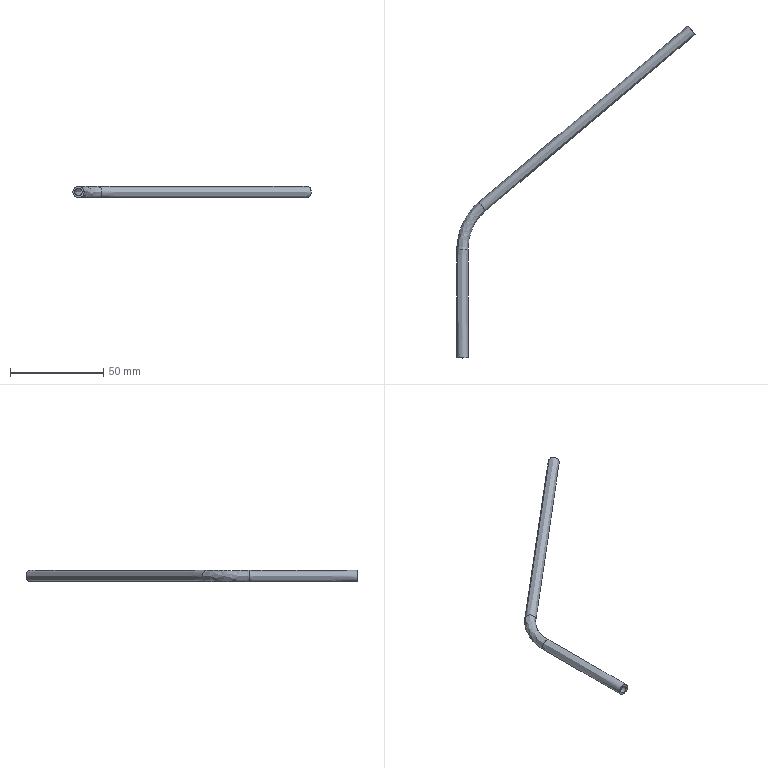Part | NX | features solid 2 | 1 solid | 8 faces | box 128.059 x 178.397 x 6 mm | volume 3604 mm3 | spline 6 | plane 2